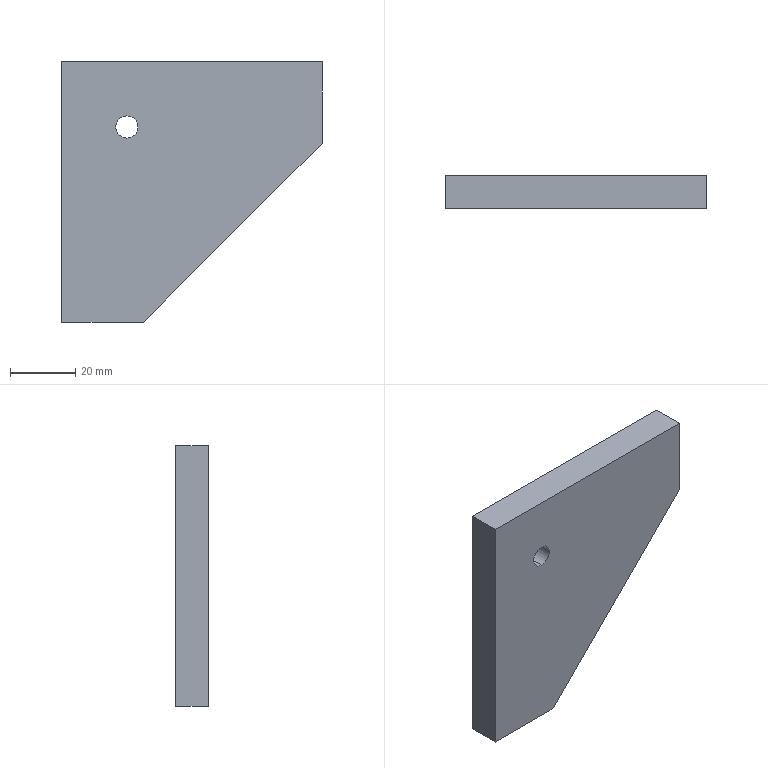Part | STEP file | 1 solid | 9 faces | box 80 x 10 x 80 mm | volume 48512 mm3 | plane 7 | cylinder 2 | commonest cylinder face diameters 6.8 x2
STEP:
#1=CARTESIAN_POINT('',(0.,0.,0.));
#2=DIRECTION('',(0.,0.,1.));
#3=DIRECTION('',(1.,0.,0.));
#4=AXIS2_PLACEMENT_3D('',#1,#2,#3);
#5=CARTESIAN_POINT('',(-20.,0.,23.4));
#6=VERTEX_POINT('',#5);
#7=CARTESIAN_POINT('',(-20.,10.,23.4));
#8=VERTEX_POINT('',#7);
#9=CARTESIAN_POINT('',(-20.,0.,23.4));
#10=DIRECTION('',(0.,1.,0.));
#11=VECTOR('',#10,1.);
#12=LINE('',#9,#11);
#13=CARTESIAN_POINT('',(-20.,0.,20.));
#14=DIRECTION('',(0.,1.,0.));
#15=DIRECTION('',(0.,0.,1.));
#16=AXIS2_PLACEMENT_3D('',#13,#14,#15);
#17=CYLINDRICAL_SURFACE('',#16,3.4);
#18=CARTESIAN_POINT('',(6.283,0.));
#19=DIRECTION('',(0.,1.));
#20=VECTOR('',#19,1.);
#21=LINE('',#18,#20);
#22=(GEOMETRIC_REPRESENTATION_CONTEXT(2)PARAMETRIC_REPRESENTATION_CONTEXT()REPRESENTATION_CONTEXT('',''));
#23=DEFINITIONAL_REPRESENTATION('',(#21),#22);
#24=PCURVE('',#17,#23);
#25=CARTESIAN_POINT('',(-20.,0.,20.));
#26=DIRECTION('',(0.,1.,0.));
#27=DIRECTION('',(0.,0.,1.));
#28=AXIS2_PLACEMENT_3D('',#25,#26,#27);
#29=CYLINDRICAL_SURFACE('',#28,3.4);
#30=CARTESIAN_POINT('',(0.,0.));
#31=DIRECTION('',(0.,1.));
#32=VECTOR('',#31,1.);
#33=LINE('',#30,#32);
#34=(GEOMETRIC_REPRESENTATION_CONTEXT(2)PARAMETRIC_REPRESENTATION_CONTEXT()REPRESENTATION_CONTEXT('',''));
#35=DEFINITIONAL_REPRESENTATION('',(#33),#34);
#36=PCURVE('',#29,#35);
#37=SURFACE_CURVE('',#12,(#24,#36),.PCURVE_S1.);
#38=EDGE_CURVE('',#6,#8,#37,.T.);
#39=ORIENTED_EDGE('',*,*,#38,.T.);
#40=CARTESIAN_POINT('',(-20.,10.,16.6));
#41=VERTEX_POINT('',#40);
#42=CARTESIAN_POINT('',(-20.,10.,20.));
#43=DIRECTION('',(0.,1.,0.));
#44=DIRECTION('',(0.,0.,1.));
#45=AXIS2_PLACEMENT_3D('',#42,#43,#44);
#46=CIRCLE('',#45,3.4);
#47=CARTESIAN_POINT('',(0.,10.));
#48=DIRECTION('',(1.,0.));
#49=VECTOR('',#48,1.);
#50=LINE('',#47,#49);
#51=(GEOMETRIC_REPRESENTATION_CONTEXT(2)PARAMETRIC_REPRESENTATION_CONTEXT()REPRESENTATION_CONTEXT('',''));
#52=DEFINITIONAL_REPRESENTATION('',(#50),#51);
#53=PCURVE('',#17,#52);
#54=CARTESIAN_POINT('',(-40.,10.,40.));
#55=DIRECTION('',(0.,-1.,0.));
#56=DIRECTION('',(0.,0.,-1.));
#57=AXIS2_PLACEMENT_3D('',#54,#55,#56);
#58=PLANE('',#57);
#59=CARTESIAN_POINT('',(16.6,20.));
#60=CARTESIAN_POINT('',(16.6,25.889));
#61=CARTESIAN_POINT('',(21.7,22.944));
#62=CARTESIAN_POINT('',(26.8,20.));
#63=CARTESIAN_POINT('',(21.7,17.056));
#64=CARTESIAN_POINT('',(16.6,14.111));
#65=CARTESIAN_POINT('',(16.6,20.));
#66=(BOUNDED_CURVE()B_SPLINE_CURVE(2,(#59,#60,#61,#62,#63,#64,#65),.UNSPECIFIED.,.T.,.F.)B_SPLINE_CURVE_WITH_KNOTS((1,2,2,2,2,1),(-2.094,0.,2.094,4.189,6.283,8.378),.UNSPECIFIED.)CURVE()GEOMETRIC_REPRESENTATION_ITEM()RATIONAL_B_SPLINE_CURVE((1.,0.5,1.,0.5,1.,0.5,1.))REPRESENTATION_ITEM(''));
#67=(GEOMETRIC_REPRESENTATION_CONTEXT(2)PARAMETRIC_REPRESENTATION_CONTEXT()REPRESENTATION_CONTEXT('',''));
#68=DEFINITIONAL_REPRESENTATION('',(#66),#67);
#69=PCURVE('',#58,#68);
#70=SURFACE_CURVE('',#46,(#53,#69),.PCURVE_S1.);
#71=EDGE_CURVE('',#41,#8,#70,.T.);
#72=ORIENTED_EDGE('',*,*,#71,.F.);
#73=CARTESIAN_POINT('',(-20.,0.,16.6));
#74=VERTEX_POINT('',#73);
#75=CARTESIAN_POINT('',(-20.,0.,16.6));
#76=DIRECTION('',(0.,1.,0.));
#77=VECTOR('',#76,1.);
#78=LINE('',#75,#77);
#79=CARTESIAN_POINT('',(3.142,0.));
#80=DIRECTION('',(0.,1.));
#81=VECTOR('',#80,1.);
#82=LINE('',#79,#81);
#83=(GEOMETRIC_REPRESENTATION_CONTEXT(2)PARAMETRIC_REPRESENTATION_CONTEXT()REPRESENTATION_CONTEXT('',''));
#84=DEFINITIONAL_REPRESENTATION('',(#82),#83);
#85=PCURVE('',#17,#84);
#86=CARTESIAN_POINT('',(3.142,0.));
#87=DIRECTION('',(0.,1.));
#88=VECTOR('',#87,1.);
#89=LINE('',#86,#88);
#90=(GEOMETRIC_REPRESENTATION_CONTEXT(2)PARAMETRIC_REPRESENTATION_CONTEXT()REPRESENTATION_CONTEXT('',''));
#91=DEFINITIONAL_REPRESENTATION('',(#89),#90);
#92=PCURVE('',#29,#91);
#93=SURFACE_CURVE('',#78,(#85,#92),.PCURVE_S1.);
#94=EDGE_CURVE('',#74,#41,#93,.T.);
#95=ORIENTED_EDGE('',*,*,#94,.F.);
#96=CARTESIAN_POINT('',(-20.,0.,20.));
#97=DIRECTION('',(0.,-1.,0.));
#98=DIRECTION('',(0.,0.,1.));
#99=AXIS2_PLACEMENT_3D('',#96,#97,#98);
#100=CIRCLE('',#99,3.4);
#101=CARTESIAN_POINT('',(6.283,0.));
#102=DIRECTION('',(-1.,0.));
#103=VECTOR('',#102,1.);
#104=LINE('',#101,#103);
#105=(GEOMETRIC_REPRESENTATION_CONTEXT(2)PARAMETRIC_REPRESENTATION_CONTEXT()REPRESENTATION_CONTEXT('',''));
#106=DEFINITIONAL_REPRESENTATION('',(#104),#105);
#107=PCURVE('',#17,#106);
#108=CARTESIAN_POINT('',(-40.,0.,40.));
#109=DIRECTION('',(0.,-1.,0.));
#110=DIRECTION('',(0.,0.,-1.));
#111=AXIS2_PLACEMENT_3D('',#108,#109,#110);
#112=PLANE('',#111);
#113=CARTESIAN_POINT('',(20.,20.));
#114=DIRECTION('',(-1.,0.));
#115=AXIS2_PLACEMENT_2D('',#113,#114);
#116=CIRCLE('',#115,3.4);
#117=(GEOMETRIC_REPRESENTATION_CONTEXT(2)PARAMETRIC_REPRESENTATION_CONTEXT()REPRESENTATION_CONTEXT('',''));
#118=DEFINITIONAL_REPRESENTATION('',(#116),#117);
#119=PCURVE('',#112,#118);
#120=SURFACE_CURVE('',#100,(#107,#119),.PCURVE_S1.);
#121=EDGE_CURVE('',#6,#74,#120,.T.);
#122=ORIENTED_EDGE('',*,*,#121,.F.);
#123=EDGE_LOOP('',(#39,#72,#95,#122));
#124=FACE_BOUND('',#123,.F.);
#125=ADVANCED_FACE('',(#124),#17,.F.);
#126=CARTESIAN_POINT('',(-20.,10.,20.));
#127=DIRECTION('',(0.,1.,0.));
#128=DIRECTION('',(0.,0.,1.));
#129=AXIS2_PLACEMENT_3D('',#126,#127,#128);
#130=CIRCLE('',#129,3.4);
#131=CARTESIAN_POINT('',(0.,10.));
#132=DIRECTION('',(1.,0.));
#133=VECTOR('',#132,1.);
#134=LINE('',#131,#133);
#135=(GEOMETRIC_REPRESENTATION_CONTEXT(2)PARAMETRIC_REPRESENTATION_CONTEXT()REPRESENTATION_CONTEXT('',''));
#136=DEFINITIONAL_REPRESENTATION('',(#134),#135);
#137=PCURVE('',#29,#136);
#138=CARTESIAN_POINT('',(16.6,20.));
#139=CARTESIAN_POINT('',(16.6,25.889));
#140=CARTESIAN_POINT('',(21.7,22.944));
#141=CARTESIAN_POINT('',(26.8,20.));
#142=CARTESIAN_POINT('',(21.7,17.056));
#143=CARTESIAN_POINT('',(16.6,14.111));
#144=CARTESIAN_POINT('',(16.6,20.));
#145=(BOUNDED_CURVE()B_SPLINE_CURVE(2,(#138,#139,#140,#141,#142,#143,#144),.UNSPECIFIED.,.T.,.F.)B_SPLINE_CURVE_WITH_KNOTS((1,2,2,2,2,1),(-2.094,0.,2.094,4.189,6.283,8.378),.UNSPECIFIED.)CURVE()GEOMETRIC_REPRESENTATION_ITEM()RATIONAL_B_SPLINE_CURVE((1.,0.5,1.,0.5,1.,0.5,1.))REPRESENTATION_ITEM(''));
#146=(GEOMETRIC_REPRESENTATION_CONTEXT(2)PARAMETRIC_REPRESENTATION_CONTEXT()REPRESENTATION_CONTEXT('',''));
#147=DEFINITIONAL_REPRESENTATION('',(#145),#146);
#148=PCURVE('',#58,#147);
#149=SURFACE_CURVE('',#130,(#137,#148),.PCURVE_S1.);
#150=EDGE_CURVE('',#8,#41,#149,.T.);
#151=ORIENTED_EDGE('',*,*,#150,.F.);
#152=ORIENTED_EDGE('',*,*,#38,.F.);
#153=CARTESIAN_POINT('',(-20.,0.,20.));
#154=DIRECTION('',(0.,-1.,0.));
#155=DIRECTION('',(0.,0.,1.));
#156=AXIS2_PLACEMENT_3D('',#153,#154,#155);
#157=CIRCLE('',#156,3.4);
#158=CARTESIAN_POINT('',(6.283,0.));
#159=DIRECTION('',(-1.,0.));
#160=VECTOR('',#159,1.);
#161=LINE('',#158,#160);
#162=(GEOMETRIC_REPRESENTATION_CONTEXT(2)PARAMETRIC_REPRESENTATION_CONTEXT()REPRESENTATION_CONTEXT('',''));
#163=DEFINITIONAL_REPRESENTATION('',(#161),#162);
#164=PCURVE('',#29,#163);
#165=CARTESIAN_POINT('',(20.,20.));
#166=DIRECTION('',(-1.,0.));
#167=AXIS2_PLACEMENT_2D('',#165,#166);
#168=CIRCLE('',#167,3.4);
#169=(GEOMETRIC_REPRESENTATION_CONTEXT(2)PARAMETRIC_REPRESENTATION_CONTEXT()REPRESENTATION_CONTEXT('',''));
#170=DEFINITIONAL_REPRESENTATION('',(#168),#169);
#171=PCURVE('',#112,#170);
#172=SURFACE_CURVE('',#157,(#164,#171),.PCURVE_S1.);
#173=EDGE_CURVE('',#74,#6,#172,.T.);
#174=ORIENTED_EDGE('',*,*,#173,.F.);
#175=ORIENTED_EDGE('',*,*,#94,.T.);
#176=EDGE_LOOP('',(#151,#152,#174,#175));
#177=FACE_BOUND('',#176,.F.);
#178=ADVANCED_FACE('',(#177),#29,.F.);
#179=ORIENTED_EDGE('',*,*,#150,.F.);
#180=ORIENTED_EDGE('',*,*,#71,.F.);
#181=EDGE_LOOP('',(#179,#180));
#182=FACE_BOUND('',#181,.T.);
#183=CARTESIAN_POINT('',(-15.,10.,-40.));
#184=VERTEX_POINT('',#183);
#185=CARTESIAN_POINT('',(40.,10.,15.));
#186=VERTEX_POINT('',#185);
#187=CARTESIAN_POINT('',(-15.,10.,-40.));
#188=DIRECTION('',(0.7071,0.,0.7071));
#189=VECTOR('',#188,1.);
#190=LINE('',#187,#189);
#191=CARTESIAN_POINT('',(80.,25.));
#192=DIRECTION('',(-0.7071,0.7071));
#193=VECTOR('',#192,1.);
#194=LINE('',#191,#193);
#195=(GEOMETRIC_REPRESENTATION_CONTEXT(2)PARAMETRIC_REPRESENTATION_CONTEXT()REPRESENTATION_CONTEXT('',''));
#196=DEFINITIONAL_REPRESENTATION('',(#194),#195);
#197=PCURVE('',#58,#196);
#198=CARTESIAN_POINT('',(-15.,0.,-40.));
#199=DIRECTION('',(-0.7071,0.,0.7071));
#200=DIRECTION('',(0.7071,0.,0.7071));
#201=AXIS2_PLACEMENT_3D('',#198,#199,#200);
#202=PLANE('',#201);
#203=CARTESIAN_POINT('',(0.,10.));
#204=DIRECTION('',(1.,0.));
#205=VECTOR('',#204,1.);
#206=LINE('',#203,#205);
#207=(GEOMETRIC_REPRESENTATION_CONTEXT(2)PARAMETRIC_REPRESENTATION_CONTEXT()REPRESENTATION_CONTEXT('',''));
#208=DEFINITIONAL_REPRESENTATION('',(#206),#207);
#209=PCURVE('',#202,#208);
#210=SURFACE_CURVE('',#190,(#197,#209),.PCURVE_S1.);
#211=EDGE_CURVE('',#184,#186,#210,.T.);
#212=ORIENTED_EDGE('',*,*,#211,.F.);
#213=CARTESIAN_POINT('',(-40.,10.,-40.));
#214=VERTEX_POINT('',#213);
#215=CARTESIAN_POINT('',(0.,10.,-40.));
#216=DIRECTION('',(1.,0.,0.));
#217=VECTOR('',#216,1.);
#218=LINE('',#215,#217);
#219=CARTESIAN_POINT('',(80.,40.));
#220=DIRECTION('',(0.,1.));
#221=VECTOR('',#220,1.);
#222=LINE('',#219,#221);
#223=(GEOMETRIC_REPRESENTATION_CONTEXT(2)PARAMETRIC_REPRESENTATION_CONTEXT()REPRESENTATION_CONTEXT('',''));
#224=DEFINITIONAL_REPRESENTATION('',(#222),#223);
#225=PCURVE('',#58,#224);
#226=CARTESIAN_POINT('',(-40.,0.,-40.));
#227=DIRECTION('',(0.,0.,1.));
#228=DIRECTION('',(1.,0.,0.));
#229=AXIS2_PLACEMENT_3D('',#226,#227,#228);
#230=PLANE('',#229);
#231=CARTESIAN_POINT('',(40.,10.));
#232=DIRECTION('',(1.,0.));
#233=VECTOR('',#232,1.);
#234=LINE('',#231,#233);
#235=(GEOMETRIC_REPRESENTATION_CONTEXT(2)PARAMETRIC_REPRESENTATION_CONTEXT()REPRESENTATION_CONTEXT('',''));
#236=DEFINITIONAL_REPRESENTATION('',(#234),#235);
#237=PCURVE('',#230,#236);
#238=SURFACE_CURVE('',#218,(#225,#237),.PCURVE_S1.);
#239=EDGE_CURVE('',#214,#184,#238,.T.);
#240=ORIENTED_EDGE('',*,*,#239,.F.);
#241=CARTESIAN_POINT('',(-40.,10.,40.));
#242=VERTEX_POINT('',#241);
#243=CARTESIAN_POINT('',(-40.,10.,0.));
#244=DIRECTION('',(0.,0.,-1.));
#245=VECTOR('',#244,1.);
#246=LINE('',#243,#245);
#247=CARTESIAN_POINT('',(40.,0.));
#248=DIRECTION('',(1.,0.));
#249=VECTOR('',#248,1.);
#250=LINE('',#247,#249);
#251=(GEOMETRIC_REPRESENTATION_CONTEXT(2)PARAMETRIC_REPRESENTATION_CONTEXT()REPRESENTATION_CONTEXT('',''));
#252=DEFINITIONAL_REPRESENTATION('',(#250),#251);
#253=PCURVE('',#58,#252);
#254=CARTESIAN_POINT('',(-40.,0.,40.));
#255=DIRECTION('',(1.,0.,0.));
#256=DIRECTION('',(0.,0.,-1.));
#257=AXIS2_PLACEMENT_3D('',#254,#255,#256);
#258=PLANE('',#257);
#259=CARTESIAN_POINT('',(40.,10.));
#260=DIRECTION('',(1.,0.));
#261=VECTOR('',#260,1.);
#262=LINE('',#259,#261);
#263=(GEOMETRIC_REPRESENTATION_CONTEXT(2)PARAMETRIC_REPRESENTATION_CONTEXT()REPRESENTATION_CONTEXT('',''));
#264=DEFINITIONAL_REPRESENTATION('',(#262),#263);
#265=PCURVE('',#258,#264);
#266=SURFACE_CURVE('',#246,(#253,#265),.PCURVE_S1.);
#267=EDGE_CURVE('',#242,#214,#266,.T.);
#268=ORIENTED_EDGE('',*,*,#267,.F.);
#269=CARTESIAN_POINT('',(40.,10.,40.));
#270=VERTEX_POINT('',#269);
#271=CARTESIAN_POINT('',(0.,10.,40.));
#272=DIRECTION('',(-1.,0.,0.));
#273=VECTOR('',#272,1.);
#274=LINE('',#271,#273);
#275=CARTESIAN_POINT('',(0.,40.));
#276=DIRECTION('',(0.,-1.));
#277=VECTOR('',#276,1.);
#278=LINE('',#275,#277);
#279=(GEOMETRIC_REPRESENTATION_CONTEXT(2)PARAMETRIC_REPRESENTATION_CONTEXT()REPRESENTATION_CONTEXT('',''));
#280=DEFINITIONAL_REPRESENTATION('',(#278),#279);
#281=PCURVE('',#58,#280);
#282=CARTESIAN_POINT('',(40.,0.,40.));
#283=DIRECTION('',(0.,0.,-1.));
#284=DIRECTION('',(-1.,0.,0.));
#285=AXIS2_PLACEMENT_3D('',#282,#283,#284);
#286=PLANE('',#285);
#287=CARTESIAN_POINT('',(40.,10.));
#288=DIRECTION('',(1.,0.));
#289=VECTOR('',#288,1.);
#290=LINE('',#287,#289);
#291=(GEOMETRIC_REPRESENTATION_CONTEXT(2)PARAMETRIC_REPRESENTATION_CONTEXT()REPRESENTATION_CONTEXT('',''));
#292=DEFINITIONAL_REPRESENTATION('',(#290),#291);
#293=PCURVE('',#286,#292);
#294=SURFACE_CURVE('',#274,(#281,#293),.PCURVE_S1.);
#295=EDGE_CURVE('',#270,#242,#294,.T.);
#296=ORIENTED_EDGE('',*,*,#295,.F.);
#297=CARTESIAN_POINT('',(40.,10.,0.));
#298=DIRECTION('',(0.,0.,1.));
#299=VECTOR('',#298,1.);
#300=LINE('',#297,#299);
#301=CARTESIAN_POINT('',(40.,80.));
#302=DIRECTION('',(-1.,0.));
#303=VECTOR('',#302,1.);
#304=LINE('',#301,#303);
#305=(GEOMETRIC_REPRESENTATION_CONTEXT(2)PARAMETRIC_REPRESENTATION_CONTEXT()REPRESENTATION_CONTEXT('',''));
#306=DEFINITIONAL_REPRESENTATION('',(#304),#305);
#307=PCURVE('',#58,#306);
#308=CARTESIAN_POINT('',(40.,0.,15.));
#309=DIRECTION('',(-1.,0.,0.));
#310=DIRECTION('',(0.,0.,1.));
#311=AXIS2_PLACEMENT_3D('',#308,#309,#310);
#312=PLANE('',#311);
#313=CARTESIAN_POINT('',(-15.,10.));
#314=DIRECTION('',(1.,0.));
#315=VECTOR('',#314,1.);
#316=LINE('',#313,#315);
#317=(GEOMETRIC_REPRESENTATION_CONTEXT(2)PARAMETRIC_REPRESENTATION_CONTEXT()REPRESENTATION_CONTEXT('',''));
#318=DEFINITIONAL_REPRESENTATION('',(#316),#317);
#319=PCURVE('',#312,#318);
#320=SURFACE_CURVE('',#300,(#307,#319),.PCURVE_S1.);
#321=EDGE_CURVE('',#186,#270,#320,.T.);
#322=ORIENTED_EDGE('',*,*,#321,.F.);
#323=EDGE_LOOP('',(#212,#240,#268,#296,#322));
#324=FACE_BOUND('',#323,.T.);
#325=ADVANCED_FACE('',(#182,#324),#58,.F.);
#326=ORIENTED_EDGE('',*,*,#121,.F.);
#327=ORIENTED_EDGE('',*,*,#173,.F.);
#328=EDGE_LOOP('',(#326,#327));
#329=FACE_BOUND('',#328,.T.);
#330=CARTESIAN_POINT('',(40.,0.,40.));
#331=VERTEX_POINT('',#330);
#332=CARTESIAN_POINT('',(-40.,0.,40.));
#333=VERTEX_POINT('',#332);
#334=CARTESIAN_POINT('',(0.,0.,40.));
#335=DIRECTION('',(-1.,0.,0.));
#336=VECTOR('',#335,1.);
#337=LINE('',#334,#336);
#338=CARTESIAN_POINT('',(0.,40.));
#339=DIRECTION('',(0.,-1.));
#340=VECTOR('',#339,1.);
#341=LINE('',#338,#340);
#342=(GEOMETRIC_REPRESENTATION_CONTEXT(2)PARAMETRIC_REPRESENTATION_CONTEXT()REPRESENTATION_CONTEXT('',''));
#343=DEFINITIONAL_REPRESENTATION('',(#341),#342);
#344=PCURVE('',#112,#343);
#345=CARTESIAN_POINT('',(40.,0.));
#346=DIRECTION('',(1.,0.));
#347=VECTOR('',#346,1.);
#348=LINE('',#345,#347);
#349=(GEOMETRIC_REPRESENTATION_CONTEXT(2)PARAMETRIC_REPRESENTATION_CONTEXT()REPRESENTATION_CONTEXT('',''));
#350=DEFINITIONAL_REPRESENTATION('',(#348),#349);
#351=PCURVE('',#286,#350);
#352=SURFACE_CURVE('',#337,(#344,#351),.PCURVE_S1.);
#353=EDGE_CURVE('',#331,#333,#352,.T.);
#354=ORIENTED_EDGE('',*,*,#353,.T.);
#355=CARTESIAN_POINT('',(-40.,0.,-40.));
#356=VERTEX_POINT('',#355);
#357=CARTESIAN_POINT('',(-40.,0.,0.));
#358=DIRECTION('',(0.,0.,-1.));
#359=VECTOR('',#358,1.);
#360=LINE('',#357,#359);
#361=CARTESIAN_POINT('',(40.,0.));
#362=DIRECTION('',(1.,0.));
#363=VECTOR('',#362,1.);
#364=LINE('',#361,#363);
#365=(GEOMETRIC_REPRESENTATION_CONTEXT(2)PARAMETRIC_REPRESENTATION_CONTEXT()REPRESENTATION_CONTEXT('',''));
#366=DEFINITIONAL_REPRESENTATION('',(#364),#365);
#367=PCURVE('',#112,#366);
#368=CARTESIAN_POINT('',(40.,0.));
#369=DIRECTION('',(1.,0.));
#370=VECTOR('',#369,1.);
#371=LINE('',#368,#370);
#372=(GEOMETRIC_REPRESENTATION_CONTEXT(2)PARAMETRIC_REPRESENTATION_CONTEXT()REPRESENTATION_CONTEXT('',''));
#373=DEFINITIONAL_REPRESENTATION('',(#371),#372);
#374=PCURVE('',#258,#373);
#375=SURFACE_CURVE('',#360,(#367,#374),.PCURVE_S1.);
#376=EDGE_CURVE('',#333,#356,#375,.T.);
#377=ORIENTED_EDGE('',*,*,#376,.T.);
#378=CARTESIAN_POINT('',(-15.,0.,-40.));
#379=VERTEX_POINT('',#378);
#380=CARTESIAN_POINT('',(0.,0.,-40.));
#381=DIRECTION('',(1.,0.,0.));
#382=VECTOR('',#381,1.);
#383=LINE('',#380,#382);
#384=CARTESIAN_POINT('',(80.,40.));
#385=DIRECTION('',(0.,1.));
#386=VECTOR('',#385,1.);
#387=LINE('',#384,#386);
#388=(GEOMETRIC_REPRESENTATION_CONTEXT(2)PARAMETRIC_REPRESENTATION_CONTEXT()REPRESENTATION_CONTEXT('',''));
#389=DEFINITIONAL_REPRESENTATION('',(#387),#388);
#390=PCURVE('',#112,#389);
#391=CARTESIAN_POINT('',(40.,0.));
#392=DIRECTION('',(1.,0.));
#393=VECTOR('',#392,1.);
#394=LINE('',#391,#393);
#395=(GEOMETRIC_REPRESENTATION_CONTEXT(2)PARAMETRIC_REPRESENTATION_CONTEXT()REPRESENTATION_CONTEXT('',''));
#396=DEFINITIONAL_REPRESENTATION('',(#394),#395);
#397=PCURVE('',#230,#396);
#398=SURFACE_CURVE('',#383,(#390,#397),.PCURVE_S1.);
#399=EDGE_CURVE('',#356,#379,#398,.T.);
#400=ORIENTED_EDGE('',*,*,#399,.T.);
#401=CARTESIAN_POINT('',(40.,0.,15.));
#402=VERTEX_POINT('',#401);
#403=CARTESIAN_POINT('',(-15.,0.,-40.));
#404=DIRECTION('',(0.7071,0.,0.7071));
#405=VECTOR('',#404,1.);
#406=LINE('',#403,#405);
#407=CARTESIAN_POINT('',(80.,25.));
#408=DIRECTION('',(-0.7071,0.7071));
#409=VECTOR('',#408,1.);
#410=LINE('',#407,#409);
#411=(GEOMETRIC_REPRESENTATION_CONTEXT(2)PARAMETRIC_REPRESENTATION_CONTEXT()REPRESENTATION_CONTEXT('',''));
#412=DEFINITIONAL_REPRESENTATION('',(#410),#411);
#413=PCURVE('',#112,#412);
#414=CARTESIAN_POINT('',(0.,0.));
#415=DIRECTION('',(1.,0.));
#416=VECTOR('',#415,1.);
#417=LINE('',#414,#416);
#418=(GEOMETRIC_REPRESENTATION_CONTEXT(2)PARAMETRIC_REPRESENTATION_CONTEXT()REPRESENTATION_CONTEXT('',''));
#419=DEFINITIONAL_REPRESENTATION('',(#417),#418);
#420=PCURVE('',#202,#419);
#421=SURFACE_CURVE('',#406,(#413,#420),.PCURVE_S1.);
#422=EDGE_CURVE('',#379,#402,#421,.T.);
#423=ORIENTED_EDGE('',*,*,#422,.T.);
#424=CARTESIAN_POINT('',(40.,0.,0.));
#425=DIRECTION('',(0.,0.,1.));
#426=VECTOR('',#425,1.);
#427=LINE('',#424,#426);
#428=CARTESIAN_POINT('',(40.,80.));
#429=DIRECTION('',(-1.,0.));
#430=VECTOR('',#429,1.);
#431=LINE('',#428,#430);
#432=(GEOMETRIC_REPRESENTATION_CONTEXT(2)PARAMETRIC_REPRESENTATION_CONTEXT()REPRESENTATION_CONTEXT('',''));
#433=DEFINITIONAL_REPRESENTATION('',(#431),#432);
#434=PCURVE('',#112,#433);
#435=CARTESIAN_POINT('',(-15.,0.));
#436=DIRECTION('',(1.,0.));
#437=VECTOR('',#436,1.);
#438=LINE('',#435,#437);
#439=(GEOMETRIC_REPRESENTATION_CONTEXT(2)PARAMETRIC_REPRESENTATION_CONTEXT()REPRESENTATION_CONTEXT('',''));
#440=DEFINITIONAL_REPRESENTATION('',(#438),#439);
#441=PCURVE('',#312,#440);
#442=SURFACE_CURVE('',#427,(#434,#441),.PCURVE_S1.);
#443=EDGE_CURVE('',#402,#331,#442,.T.);
#444=ORIENTED_EDGE('',*,*,#443,.T.);
#445=EDGE_LOOP('',(#354,#377,#400,#423,#444));
#446=FACE_BOUND('',#445,.T.);
#447=ADVANCED_FACE('',(#329,#446),#112,.T.);
#448=CARTESIAN_POINT('',(40.,5.,15.));
#449=DIRECTION('',(0.,-1.,0.));
#450=VECTOR('',#449,1.);
#451=LINE('',#448,#450);
#452=CARTESIAN_POINT('',(0.,5.));
#453=DIRECTION('',(0.,-1.));
#454=VECTOR('',#453,1.);
#455=LINE('',#452,#454);
#456=(GEOMETRIC_REPRESENTATION_CONTEXT(2)PARAMETRIC_REPRESENTATION_CONTEXT()REPRESENTATION_CONTEXT('',''));
#457=DEFINITIONAL_REPRESENTATION('',(#455),#456);
#458=PCURVE('',#312,#457);
#459=CARTESIAN_POINT('',(77.782,5.));
#460=DIRECTION('',(0.,-1.));
#461=VECTOR('',#460,1.);
#462=LINE('',#459,#461);
#463=(GEOMETRIC_REPRESENTATION_CONTEXT(2)PARAMETRIC_REPRESENTATION_CONTEXT()REPRESENTATION_CONTEXT('',''));
#464=DEFINITIONAL_REPRESENTATION('',(#462),#463);
#465=PCURVE('',#202,#464);
#466=SURFACE_CURVE('',#451,(#458,#465),.PCURVE_S1.);
#467=EDGE_CURVE('',#186,#402,#466,.T.);
#468=ORIENTED_EDGE('',*,*,#467,.F.);
#469=ORIENTED_EDGE('',*,*,#321,.T.);
#470=CARTESIAN_POINT('',(40.,5.,40.));
#471=DIRECTION('',(0.,1.,0.));
#472=VECTOR('',#471,1.);
#473=LINE('',#470,#472);
#474=CARTESIAN_POINT('',(25.,5.));
#475=DIRECTION('',(0.,1.));
#476=VECTOR('',#475,1.);
#477=LINE('',#474,#476);
#478=(GEOMETRIC_REPRESENTATION_CONTEXT(2)PARAMETRIC_REPRESENTATION_CONTEXT()REPRESENTATION_CONTEXT('',''));
#479=DEFINITIONAL_REPRESENTATION('',(#477),#478);
#480=PCURVE('',#312,#479);
#481=CARTESIAN_POINT('',(0.,5.));
#482=DIRECTION('',(0.,1.));
#483=VECTOR('',#482,1.);
#484=LINE('',#481,#483);
#485=(GEOMETRIC_REPRESENTATION_CONTEXT(2)PARAMETRIC_REPRESENTATION_CONTEXT()REPRESENTATION_CONTEXT('',''));
#486=DEFINITIONAL_REPRESENTATION('',(#484),#485);
#487=PCURVE('',#286,#486);
#488=SURFACE_CURVE('',#473,(#480,#487),.PCURVE_S1.);
#489=EDGE_CURVE('',#331,#270,#488,.T.);
#490=ORIENTED_EDGE('',*,*,#489,.F.);
#491=ORIENTED_EDGE('',*,*,#443,.F.);
#492=EDGE_LOOP('',(#468,#469,#490,#491));
#493=FACE_BOUND('',#492,.T.);
#494=ADVANCED_FACE('',(#493),#312,.F.);
#495=ORIENTED_EDGE('',*,*,#467,.T.);
#496=ORIENTED_EDGE('',*,*,#422,.F.);
#497=CARTESIAN_POINT('',(-15.,5.,-40.));
#498=DIRECTION('',(0.,-1.,0.));
#499=VECTOR('',#498,1.);
#500=LINE('',#497,#499);
#501=CARTESIAN_POINT('',(0.,5.));
#502=DIRECTION('',(0.,-1.));
#503=VECTOR('',#502,1.);
#504=LINE('',#501,#503);
#505=(GEOMETRIC_REPRESENTATION_CONTEXT(2)PARAMETRIC_REPRESENTATION_CONTEXT()REPRESENTATION_CONTEXT('',''));
#506=DEFINITIONAL_REPRESENTATION('',(#504),#505);
#507=PCURVE('',#202,#506);
#508=CARTESIAN_POINT('',(25.,5.));
#509=DIRECTION('',(0.,-1.));
#510=VECTOR('',#509,1.);
#511=LINE('',#508,#510);
#512=(GEOMETRIC_REPRESENTATION_CONTEXT(2)PARAMETRIC_REPRESENTATION_CONTEXT()REPRESENTATION_CONTEXT('',''));
#513=DEFINITIONAL_REPRESENTATION('',(#511),#512);
#514=PCURVE('',#230,#513);
#515=SURFACE_CURVE('',#500,(#507,#514),.PCURVE_S1.);
#516=EDGE_CURVE('',#184,#379,#515,.T.);
#517=ORIENTED_EDGE('',*,*,#516,.F.);
#518=ORIENTED_EDGE('',*,*,#211,.T.);
#519=EDGE_LOOP('',(#495,#496,#517,#518));
#520=FACE_BOUND('',#519,.T.);
#521=ADVANCED_FACE('',(#520),#202,.F.);
#522=ORIENTED_EDGE('',*,*,#516,.T.);
#523=ORIENTED_EDGE('',*,*,#399,.F.);
#524=CARTESIAN_POINT('',(-40.,5.,-40.));
#525=DIRECTION('',(0.,-1.,0.));
#526=VECTOR('',#525,1.);
#527=LINE('',#524,#526);
#528=CARTESIAN_POINT('',(0.,5.));
#529=DIRECTION('',(0.,-1.));
#530=VECTOR('',#529,1.);
#531=LINE('',#528,#530);
#532=(GEOMETRIC_REPRESENTATION_CONTEXT(2)PARAMETRIC_REPRESENTATION_CONTEXT()REPRESENTATION_CONTEXT('',''));
#533=DEFINITIONAL_REPRESENTATION('',(#531),#532);
#534=PCURVE('',#230,#533);
#535=CARTESIAN_POINT('',(80.,5.));
#536=DIRECTION('',(0.,-1.));
#537=VECTOR('',#536,1.);
#538=LINE('',#535,#537);
#539=(GEOMETRIC_REPRESENTATION_CONTEXT(2)PARAMETRIC_REPRESENTATION_CONTEXT()REPRESENTATION_CONTEXT('',''));
#540=DEFINITIONAL_REPRESENTATION('',(#538),#539);
#541=PCURVE('',#258,#540);
#542=SURFACE_CURVE('',#527,(#534,#541),.PCURVE_S1.);
#543=EDGE_CURVE('',#214,#356,#542,.T.);
#544=ORIENTED_EDGE('',*,*,#543,.F.);
#545=ORIENTED_EDGE('',*,*,#239,.T.);
#546=EDGE_LOOP('',(#522,#523,#544,#545));
#547=FACE_BOUND('',#546,.T.);
#548=ADVANCED_FACE('',(#547),#230,.F.);
#549=CARTESIAN_POINT('',(-40.,5.,40.));
#550=DIRECTION('',(0.,-1.,0.));
#551=VECTOR('',#550,1.);
#552=LINE('',#549,#551);
#553=CARTESIAN_POINT('',(0.,5.));
#554=DIRECTION('',(0.,-1.));
#555=VECTOR('',#554,1.);
#556=LINE('',#553,#555);
#557=(GEOMETRIC_REPRESENTATION_CONTEXT(2)PARAMETRIC_REPRESENTATION_CONTEXT()REPRESENTATION_CONTEXT('',''));
#558=DEFINITIONAL_REPRESENTATION('',(#556),#557);
#559=PCURVE('',#258,#558);
#560=CARTESIAN_POINT('',(80.,5.));
#561=DIRECTION('',(0.,-1.));
#562=VECTOR('',#561,1.);
#563=LINE('',#560,#562);
#564=(GEOMETRIC_REPRESENTATION_CONTEXT(2)PARAMETRIC_REPRESENTATION_CONTEXT()REPRESENTATION_CONTEXT('',''));
#565=DEFINITIONAL_REPRESENTATION('',(#563),#564);
#566=PCURVE('',#286,#565);
#567=SURFACE_CURVE('',#552,(#559,#566),.PCURVE_S1.);
#568=EDGE_CURVE('',#242,#333,#567,.T.);
#569=ORIENTED_EDGE('',*,*,#568,.F.);
#570=ORIENTED_EDGE('',*,*,#267,.T.);
#571=ORIENTED_EDGE('',*,*,#543,.T.);
#572=ORIENTED_EDGE('',*,*,#376,.F.);
#573=EDGE_LOOP('',(#569,#570,#571,#572));
#574=FACE_BOUND('',#573,.T.);
#575=ADVANCED_FACE('',(#574),#258,.F.);
#576=ORIENTED_EDGE('',*,*,#489,.T.);
#577=ORIENTED_EDGE('',*,*,#295,.T.);
#578=ORIENTED_EDGE('',*,*,#568,.T.);
#579=ORIENTED_EDGE('',*,*,#353,.F.);
#580=EDGE_LOOP('',(#576,#577,#578,#579));
#581=FACE_BOUND('',#580,.T.);
#582=ADVANCED_FACE('',(#581),#286,.F.);
#583=CLOSED_SHELL('',(#125,#178,#325,#447,#494,#521,#548,#575,#582));
#584=MANIFOLD_SOLID_BREP('',#583);
#585=(LENGTH_UNIT()NAMED_UNIT(*)SI_UNIT(.MILLI.,.METRE.));
#586=UNCERTAINTY_MEASURE_WITH_UNIT(LENGTH_MEASURE(0.0000001),#585,'','');
#587=(NAMED_UNIT(*)PLANE_ANGLE_UNIT()SI_UNIT($,.RADIAN.));
#588=(NAMED_UNIT(*)SI_UNIT($,.STERADIAN.)SOLID_ANGLE_UNIT());
#589=(GEOMETRIC_REPRESENTATION_CONTEXT(3)GLOBAL_UNCERTAINTY_ASSIGNED_CONTEXT((#586))GLOBAL_UNIT_ASSIGNED_CONTEXT((#585,#587,#588))REPRESENTATION_CONTEXT('',''));
#590=ADVANCED_BREP_SHAPE_REPRESENTATION('',(#4,#584),#589);